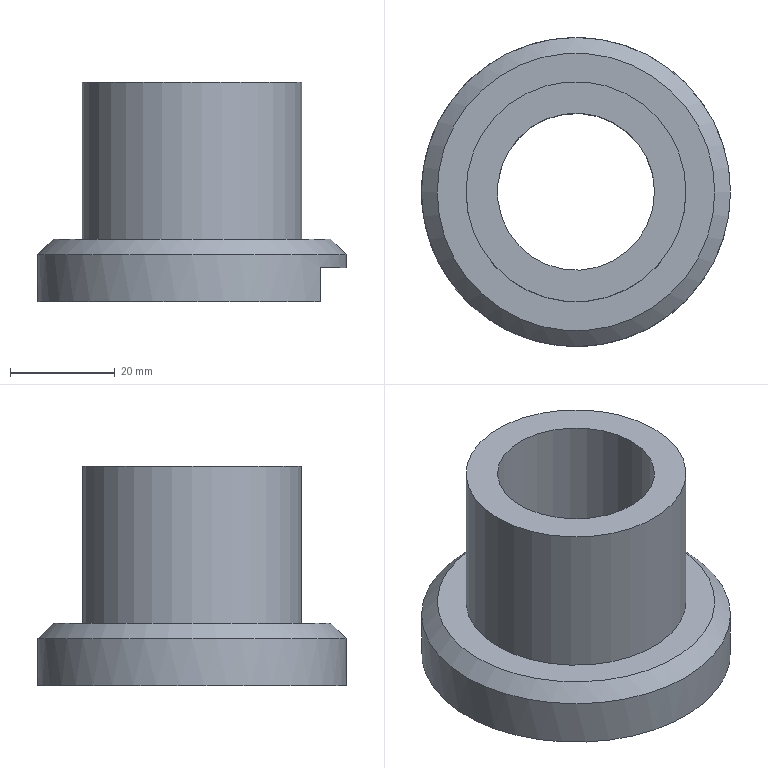Part | NX | features DATUM_CSYS 4, EXTRUDE 3, SKETCH 3, CHAMFER 1 | 1 solid | 9 faces | box 59 x 59 x 42 mm | volume 43152 mm3 | plane 5 | cylinder 3 | cone 1 | commonest cylinder face diameters 30 x1 42 x1 59 x1
STEP:
#1=CARTESIAN_POINT('',(21.,0.,30.));
#2=VERTEX_POINT('',#1);
#3=CARTESIAN_POINT('',(0.,0.,30.));
#4=DIRECTION('',(0.,0.,1.));
#5=DIRECTION('',(1.,0.,0.));
#6=AXIS2_PLACEMENT_3D('',#3,#4,#5);
#7=CIRCLE('',#6,21.);
#8=EDGE_CURVE('',#2,#2,#7,.T.);
#9=ORIENTED_EDGE('',*,*,#8,.F.);
#10=EDGE_LOOP('',(#9));
#11=FACE_BOUND('',#10,.T.);
#12=CARTESIAN_POINT('',(21.,0.,0.));
#13=VERTEX_POINT('',#12);
#14=CARTESIAN_POINT('',(0.,0.,0.));
#15=DIRECTION('',(0.,0.,1.));
#16=DIRECTION('',(1.,0.,0.));
#17=AXIS2_PLACEMENT_3D('',#14,#15,#16);
#18=CIRCLE('',#17,21.);
#19=EDGE_CURVE('',#13,#13,#18,.T.);
#20=ORIENTED_EDGE('',*,*,#19,.T.);
#21=EDGE_LOOP('',(#20));
#22=FACE_BOUND('',#21,.T.);
#23=CARTESIAN_POINT('',(0.,0.,30.));
#24=DIRECTION('',(0.,0.,-1.));
#25=DIRECTION('',(-1.,0.,0.));
#26=AXIS2_PLACEMENT_3D('',#23,#24,#25);
#27=CYLINDRICAL_SURFACE('',#26,21.);
#28=ADVANCED_FACE('',(#11,#22),#27,.T.);
#29=CARTESIAN_POINT('',(15.,0.,30.));
#30=VERTEX_POINT('',#29);
#31=CARTESIAN_POINT('',(0.,0.,30.));
#32=DIRECTION('',(0.,0.,1.));
#33=DIRECTION('',(1.,0.,0.));
#34=AXIS2_PLACEMENT_3D('',#31,#32,#33);
#35=CIRCLE('',#34,15.);
#36=EDGE_CURVE('',#30,#30,#35,.T.);
#37=ORIENTED_EDGE('',*,*,#36,.T.);
#38=EDGE_LOOP('',(#37));
#39=FACE_BOUND('',#38,.T.);
#40=CARTESIAN_POINT('',(15.,0.,-12.));
#41=VERTEX_POINT('',#40);
#42=CARTESIAN_POINT('',(0.,0.,-12.));
#43=DIRECTION('',(0.,0.,1.));
#44=DIRECTION('',(1.,0.,0.));
#45=AXIS2_PLACEMENT_3D('',#42,#43,#44);
#46=CIRCLE('',#45,15.);
#47=EDGE_CURVE('',#41,#41,#46,.T.);
#48=ORIENTED_EDGE('',*,*,#47,.F.);
#49=EDGE_LOOP('',(#48));
#50=FACE_BOUND('',#49,.T.);
#51=CARTESIAN_POINT('',(0.,0.,30.));
#52=DIRECTION('',(0.,0.,-1.));
#53=DIRECTION('',(-1.,0.,0.));
#54=AXIS2_PLACEMENT_3D('',#51,#52,#53);
#55=CYLINDRICAL_SURFACE('',#54,15.);
#56=ADVANCED_FACE('',(#39,#50),#55,.F.);
#57=ORIENTED_EDGE('',*,*,#8,.T.);
#58=EDGE_LOOP('',(#57));
#59=FACE_BOUND('',#58,.T.);
#60=ORIENTED_EDGE('',*,*,#36,.F.);
#61=EDGE_LOOP('',(#60));
#62=FACE_BOUND('',#61,.T.);
#63=CARTESIAN_POINT('',(0.,0.,30.));
#64=DIRECTION('',(0.,0.,1.));
#65=DIRECTION('',(1.,0.,0.));
#66=AXIS2_PLACEMENT_3D('',#63,#64,#65);
#67=PLANE('',#66);
#68=ADVANCED_FACE('',(#59,#62),#67,.T.);
#69=CARTESIAN_POINT('',(24.5,-16.432,-5.5));
#70=VERTEX_POINT('',#69);
#71=CARTESIAN_POINT('',(24.5,-16.432,-12.));
#72=VERTEX_POINT('',#71);
#73=CARTESIAN_POINT('',(24.5,-16.432,-12.));
#74=DIRECTION('',(0.,0.,1.));
#75=VECTOR('',#74,1000.);
#76=LINE('',#73,#75);
#77=EDGE_CURVE('',#70,#72,#76,.F.);
#78=ORIENTED_EDGE('',*,*,#77,.F.);
#79=CARTESIAN_POINT('',(24.5,16.432,-5.5));
#80=VERTEX_POINT('',#79);
#81=CARTESIAN_POINT('',(0.,0.,-5.5));
#82=DIRECTION('',(0.,0.,1.));
#83=DIRECTION('',(1.,0.,0.));
#84=AXIS2_PLACEMENT_3D('',#81,#82,#83);
#85=CIRCLE('',#84,29.5);
#86=EDGE_CURVE('',#80,#70,#85,.F.);
#87=ORIENTED_EDGE('',*,*,#86,.F.);
#88=CARTESIAN_POINT('',(24.5,16.432,-12.));
#89=VERTEX_POINT('',#88);
#90=CARTESIAN_POINT('',(24.5,16.432,-12.));
#91=DIRECTION('',(0.,0.,1.));
#92=VECTOR('',#91,1000.);
#93=LINE('',#90,#92);
#94=EDGE_CURVE('',#89,#80,#93,.T.);
#95=ORIENTED_EDGE('',*,*,#94,.F.);
#96=CARTESIAN_POINT('',(0.,0.,-12.));
#97=DIRECTION('',(0.,0.,1.));
#98=DIRECTION('',(1.,0.,0.));
#99=AXIS2_PLACEMENT_3D('',#96,#97,#98);
#100=CIRCLE('',#99,29.5);
#101=EDGE_CURVE('',#89,#72,#100,.T.);
#102=ORIENTED_EDGE('',*,*,#101,.T.);
#103=EDGE_LOOP('',(#78,#87,#95,#102));
#104=FACE_BOUND('',#103,.T.);
#105=CARTESIAN_POINT('',(29.5,0.,-3.));
#106=VERTEX_POINT('',#105);
#107=CARTESIAN_POINT('',(0.,0.,-3.));
#108=DIRECTION('',(0.,0.,1.));
#109=DIRECTION('',(1.,0.,0.));
#110=AXIS2_PLACEMENT_3D('',#107,#108,#109);
#111=CIRCLE('',#110,29.5);
#112=EDGE_CURVE('',#106,#106,#111,.F.);
#113=ORIENTED_EDGE('',*,*,#112,.T.);
#114=EDGE_LOOP('',(#113));
#115=FACE_BOUND('',#114,.T.);
#116=CARTESIAN_POINT('',(0.,0.,-12.));
#117=DIRECTION('',(0.,0.,1.));
#118=DIRECTION('',(1.,0.,0.));
#119=AXIS2_PLACEMENT_3D('',#116,#117,#118);
#120=CYLINDRICAL_SURFACE('',#119,29.5);
#121=ADVANCED_FACE('',(#104,#115),#120,.T.);
#122=ORIENTED_EDGE('',*,*,#101,.F.);
#123=CARTESIAN_POINT('',(24.5,0.,-12.));
#124=DIRECTION('',(0.,-1.,0.));
#125=VECTOR('',#124,1000.);
#126=LINE('',#123,#125);
#127=EDGE_CURVE('',#89,#72,#126,.T.);
#128=ORIENTED_EDGE('',*,*,#127,.T.);
#129=EDGE_LOOP('',(#122,#128));
#130=FACE_BOUND('',#129,.T.);
#131=ORIENTED_EDGE('',*,*,#47,.T.);
#132=EDGE_LOOP('',(#131));
#133=FACE_BOUND('',#132,.T.);
#134=CARTESIAN_POINT('',(0.,0.,-12.));
#135=DIRECTION('',(0.,0.,1.));
#136=DIRECTION('',(1.,0.,0.));
#137=AXIS2_PLACEMENT_3D('',#134,#135,#136);
#138=PLANE('',#137);
#139=ADVANCED_FACE('',(#130,#133),#138,.F.);
#140=CARTESIAN_POINT('',(26.5,0.,0.));
#141=VERTEX_POINT('',#140);
#142=CARTESIAN_POINT('',(0.,0.,0.));
#143=DIRECTION('',(0.,0.,1.));
#144=DIRECTION('',(1.,0.,0.));
#145=AXIS2_PLACEMENT_3D('',#142,#143,#144);
#146=CIRCLE('',#145,26.5);
#147=EDGE_CURVE('',#141,#141,#146,.T.);
#148=ORIENTED_EDGE('',*,*,#147,.T.);
#149=EDGE_LOOP('',(#148));
#150=FACE_BOUND('',#149,.T.);
#151=ORIENTED_EDGE('',*,*,#19,.F.);
#152=EDGE_LOOP('',(#151));
#153=FACE_BOUND('',#152,.T.);
#154=CARTESIAN_POINT('',(0.,0.,0.));
#155=DIRECTION('',(0.,0.,1.));
#156=DIRECTION('',(1.,0.,0.));
#157=AXIS2_PLACEMENT_3D('',#154,#155,#156);
#158=PLANE('',#157);
#159=ADVANCED_FACE('',(#150,#153),#158,.T.);
#160=ORIENTED_EDGE('',*,*,#112,.F.);
#161=EDGE_LOOP('',(#160));
#162=FACE_BOUND('',#161,.T.);
#163=ORIENTED_EDGE('',*,*,#147,.F.);
#164=EDGE_LOOP('',(#163));
#165=FACE_BOUND('',#164,.T.);
#166=CARTESIAN_POINT('',(0.,0.,0.));
#167=DIRECTION('',(0.,0.,-1.));
#168=DIRECTION('',(-1.,0.,0.));
#169=AXIS2_PLACEMENT_3D('',#166,#167,#168);
#170=CONICAL_SURFACE('',#169,26.5,0.7854);
#171=ADVANCED_FACE('',(#162,#165),#170,.T.);
#172=ORIENTED_EDGE('',*,*,#77,.T.);
#173=ORIENTED_EDGE('',*,*,#127,.F.);
#174=ORIENTED_EDGE('',*,*,#94,.T.);
#175=CARTESIAN_POINT('',(24.5,21.5,-5.5));
#176=DIRECTION('',(0.,-1.,0.));
#177=VECTOR('',#176,1000.);
#178=LINE('',#175,#177);
#179=EDGE_CURVE('',#70,#80,#178,.F.);
#180=ORIENTED_EDGE('',*,*,#179,.F.);
#181=EDGE_LOOP('',(#172,#173,#174,#180));
#182=FACE_BOUND('',#181,.T.);
#183=CARTESIAN_POINT('',(24.5,21.5,-12.));
#184=DIRECTION('',(-1.,0.,0.));
#185=DIRECTION('',(0.,0.,1.));
#186=AXIS2_PLACEMENT_3D('',#183,#184,#185);
#187=PLANE('',#186);
#188=ADVANCED_FACE('',(#182),#187,.F.);
#189=ORIENTED_EDGE('',*,*,#86,.T.);
#190=ORIENTED_EDGE('',*,*,#179,.T.);
#191=EDGE_LOOP('',(#189,#190));
#192=FACE_BOUND('',#191,.T.);
#193=CARTESIAN_POINT('',(0.,0.,-5.5));
#194=DIRECTION('',(0.,0.,1.));
#195=DIRECTION('',(1.,0.,0.));
#196=AXIS2_PLACEMENT_3D('',#193,#194,#195);
#197=PLANE('',#196);
#198=ADVANCED_FACE('',(#192),#197,.F.);
#199=CLOSED_SHELL('',(#28,#56,#68,#121,#139,#159,#171,#188,#198));
#200=MANIFOLD_SOLID_BREP('',#199);
#201=(LENGTH_UNIT()NAMED_UNIT(*)SI_UNIT(.MILLI.,.METRE.));
#202=UNCERTAINTY_MEASURE_WITH_UNIT(LENGTH_MEASURE(0.00001),#201,'','');
#203=(NAMED_UNIT(*)PLANE_ANGLE_UNIT()SI_UNIT($,.RADIAN.));
#204=(NAMED_UNIT(*)SI_UNIT($,.STERADIAN.)SOLID_ANGLE_UNIT());
#205=(GEOMETRIC_REPRESENTATION_CONTEXT(3)GLOBAL_UNCERTAINTY_ASSIGNED_CONTEXT((#202))GLOBAL_UNIT_ASSIGNED_CONTEXT((#201,#203,#204))REPRESENTATION_CONTEXT('',''));
#206=ADVANCED_BREP_SHAPE_REPRESENTATION('',(#200),#205);